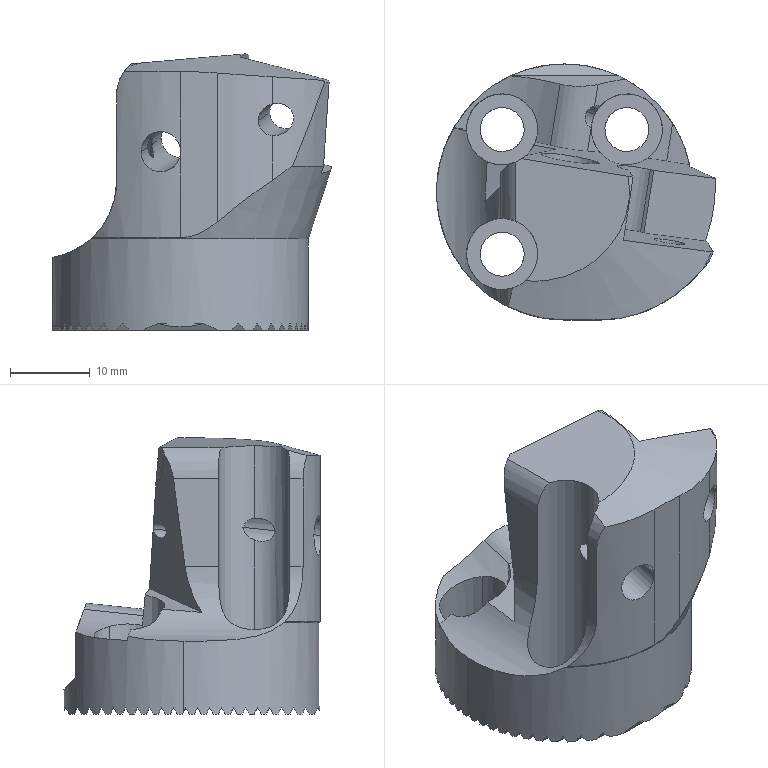CAM job | Mastercam | 3-axis milling, 5-axis milling, drilling
Tools:
tool_number,name,type,diameter_mm,corner_radius_mm,flutes,flute_length_mm,overall_length_mm,shoulder_length_mm,holder_diameter_mm,length_offset,diameter_offset,default_rpm,default_feed_mm_min,default_plunge_mm_min,coolant
1,2 Drill,drill,2,0,2,25,25,25,50,1,1,2998,359.76,600,COOL_OFF
2,6 120deg Spot Drill,drill,6,0,2,25,35,35,31.877,2,2,1000,120,600,COOL_OFF
3,4.3 Drill,drill,4.3,0,2,25,40,40,31.877,3,3,1395,167.4,600,COOL_OFF
4,12 Flat End Mill Rough,end mill,12,0,4,35,35,35,31.877,4,4,833,99.96,600,COOL_OFF
5,6 Flat End Mill Rough,end mill,6,0,4,20,20,20,31.877,5,5,1667,200.04,600,COOL_OFF
6,4 Flat End Mill Rough,end mill,4,0,4,20,20,20,27.495,6,6,2501,300.12,600,COOL_OFF
7,4 Flat End Mill Finish,end mill,4,0,4,20,20,20,27.495,7,7,2501,300.12,600,COOL_OFF
9,12 Flat End Mill Finish,end mill,12,0,4,35,35,35,31.877,9,9,833,99.96,600,COOL_OFF
10,30 Bull Nose Mill,bull end mill,30,0.8,4,25,50,25,50,10,10,400,48,600,COOL_OFF
11,4 Flat End Mill,end mill,4,0,4,20,20,20,50,11,11,2222,266.64,600,COOL_OFF
12,6 Spot Drill,drill,6,0,2,25,50,37,50,12,12,1000,120,600,COOL_OFF
13,3.3 Drill,drill,3.3,0,2,25,50,40,50,13,13,1818,218.16,600,COOL_OFF
14,3.15 Thread Mill,thread mill,3.15,0,4,2.1,20,20,31.877,14,14,1905,228.6,600,COOL_OFF
15,2.5 Ball Mill,ball end mill,2.5,1.25,4,3,20,3,31.877,15,15,4800,576,600,COOL_OFF
16,M5 x 0.8 RH Tap,drill,5,0,2,22,25,22,31.877,16,16,1200,960.0,600,COOL_OFF
17,3 Drill,drill,3,0,2,25,40,35,50,17,17,2000,240,600,COOL_OFF
18,5.5 Flat Mill,end mill,5.5,0,4,25,25,25,50,18,18,1818,218.16,600,COOL_OFF
Operations:
seq,operation,operation_type,tool_number,tool_name,tool_diameter_mm,spindle_rpm,feed_mm_min,plunge_mm_min,retract_mm_min,cycle_time_s,wcs,posted,nc_file
1,2D High Speed (2D Dynamic Mill) - [WCS: Top] - [Tplane: Top],HighSpeed2D,4,12 Flat End Mill Rough,12,3500,2500,2000,1200,17.289,Top,yes,.nc
2,2D High Speed (2D Dynamic Mill) - [WCS: Top] - [Tplane: Ins],HighSpeed2D,4,12 Flat End Mill Rough,12,3500,2500,2000,1200,118.677,Top,yes,.nc
3,Contour (2D) - [WCS: Top] - [Tplane: Ins],Contour,4,12 Flat End Mill Rough,12,3500,1000,2000,1200,7.025,Top,yes,.nc
4,Contour (Ramp) - [WCS: Top] - [Tplane: A0],Contour,4,12 Flat End Mill Rough,12,3500,1000,2000,1200,6.229,Top,yes,.nc
5,Contour (Ramp) - [WCS: Top] - [Tplane: A45],Contour,4,12 Flat End Mill Rough,12,3500,1000,2000,1200,4.179,Top,yes,.nc
6,Contour (Ramp) - [WCS: Top] - [Tplane: A-30],Contour,4,12 Flat End Mill Rough,12,3500,1000,2000,1200,4.291,Top,yes,.nc
7,2D High Speed (2D Dynamic Mill) - [WCS: Top] - [Tplane: A0-1],HighSpeed2D,4,12 Flat End Mill Rough,12,3500,2500,2000,1200,44.017,Top,yes,.nc
8,2D High Speed (2D Dynamic Mill) - [WCS: Top] - [Tplane: Ins],HighSpeed2D,5,6 Flat End Mill Rough,6,3500,1500,2000,1200,72.03,Top,yes,.nc
9,Contour (Remachining) - [WCS: Top] - [Tplane: Ins],Contour,6,4 Flat End Mill Rough,4,3500,400,2000,1200,68.934,Top,yes,.nc
10,Contour (Ramp) - [WCS: Top] - [Tplane: Ins],Contour,6,4 Flat End Mill Rough,4,3500,400,2000,1200,25.066,Top,yes,.nc
11,Contour (2D) - [WCS: Top] - [Tplane: Ins],Contour,7,4 Flat End Mill Finish,4,3500,400,2000,1200,16.515,Top,yes,.nc
12,Contour (2D) - [WCS: Top] - [Tplane: Pl-2],Contour,7,4 Flat End Mill Finish,4,3500,400,2000,1200,2.3,Top,yes,.nc
13,Contour (2D) - [WCS: Top] - [Tplane: Pl-3],Contour,7,4 Flat End Mill Finish,4,3500,400,2000,1200,2.316,Top,yes,.nc
14,Contour (2D) - [WCS: Top] - [Tplane: Top],Contour,9,12 Flat End Mill Finish,12,3500,600,2000,1200,16.491,Top,yes,.nc
15,Contour (2D) - [WCS: Top] - [Tplane: Ins],Contour,9,12 Flat End Mill Finish,12,3500,600,2000,1200,5.685,Top,yes,.nc
16,Contour (2D) - [WCS: Top] - [Tplane: A0],Contour,9,12 Flat End Mill Finish,12,3500,600,2000,1200,3.71,Top,yes,.nc
17,Contour (2D) - [WCS: Top] - [Tplane: A45],Contour,9,12 Flat End Mill Finish,12,3500,600,2000,1200,3.552,Top,yes,.nc
18,Contour (2D) - [WCS: Top] - [Tplane: A-30],Contour,9,12 Flat End Mill Finish,12,3500,600,2000,1200,3.664,Top,yes,.nc
19,Contour (2D) - [WCS: Top] - [Tplane: A0-1],Contour,9,12 Flat End Mill Finish,12,3500,600,2000,1200,6.75,Top,yes,.nc
20,Contour (2D) - [WCS: Top] - [Tplane: Ins],Contour,10,30 Bull Nose Mill,30,3500,400,2000,1200,11.272,Top,yes,.nc
21,Drill/Counterbore - [WCS: Top] - [Tplane: A0],Drill,12,6 Spot Drill,6,2000,100,5.409,5.409,1.68,Top,yes,.nc
22,Drill/Counterbore - [WCS: Top] - [Tplane: Ins],Drill,12,6 Spot Drill,6,2000,100,5.409,5.409,5.052,Top,yes,.nc
23,Peck Drill - [WCS: Top] - [Tplane: Ins],Drill,3,4.3 Drill,4.3,2500,100,600,1200,12.631,Top,yes,.nc
24,Peck Drill - [WCS: Top] - [Tplane: Ins],Drill,13,3.3 Drill,3.3,3000,60,600,1200,12.632,Top,yes,.nc
25,Peck Drill - [WCS: Top] - [Tplane: A0],Drill,13,3.3 Drill,3.3,3000,60,600,1200,13.763,Top,yes,.nc
26,Drill/Counterbore - [WCS: Top] - [Tplane: Ins],Drill,1,2 Drill,2,3000,60,600,1200,7.093,Top,yes,.nc
27,Drill/Counterbore - [WCS: Top] - [Tplane: CB],Drill,11,4 Flat End Mill,4,2000,100,600,1200,3.486,Top,yes,.nc
28,Drill/Counterbore - [WCS: Top] - [Tplane: CB],Drill,18,5.5 Flat Mill,5.5,1000,100,600,1200,4.09,Top,yes,.nc
29,Drill/Counterbore - [WCS: Top] - [Tplane: Ins],Drill,12,6 Spot Drill,6,2000,200,600,1200,1.559,Top,yes,.nc
30,Drill/Counterbore - [WCS: Top] - [Tplane: Ins],Drill,12,6 Spot Drill,6,2000,200,600,1200,1.407,Top,yes,.nc
31,Drill/Counterbore - [WCS: Top] - [Tplane: A0],Drill,12,6 Spot Drill,6,2000,200,600,1200,1.415,Top,yes,.nc
32,Thread Mill - [WCS: Top] - [Tplane: A0],ThreadMill,14,3.15 Thread Mill,3.15,3000,300,2000,1200,7.04,Top,yes,.nc
33,Stock model - [WCS: Top] - [Tplane: Top] - 2,139,,,,0,0,0,0,0,Top,no,
34,Thread Mill - [WCS: Top] - [Tplane: Ins],ThreadMill,14,3.15 Thread Mill,3.15,3000,300,2000,1200,22.324,Top,yes,.nc
35,Tap - [WCS: Top] - [Tplane: Ins],Drill,16,M5 x 0.8 RH Tap,5,200,160.0,600,1200,25.356,Top,yes,.nc
36,2D High Speed (2D Dynamic Mill) - [WCS: Top] - [Tplane: BkB],HighSpeed2D,4,12 Flat End Mill Rough,12,3500,2000,2000,1200,12.497,Top,yes,.nc
37,Contour (2D) - [WCS: Top] - [Tplane: BkB],Contour,9,12 Flat End Mill Finish,12,3500,600,2000,1200,2.75,Top,yes,.nc
38,Deburr 5-axis - [WCS: Top] - [Tplane: Top],459,15,2.5 Ball Mill,2.5,4500,1000,600,1200,7.913,Top,yes,.nc
39,Deburr 5-axis - [WCS: Top] - [Tplane: Top],459,15,2.5 Ball Mill,2.5,4500,1000,600,1200,4.558,Top,yes,.nc
40,Drill/Counterbore - [WCS: Top] - [Tplane: Outlet hole],Drill,2,6 120deg Spot Drill,6,2000,80,600,1200,2.361,Top,yes,.nc
41,Drill/Counterbore - [WCS: Top] - [Tplane: Outlet hole],Drill,17,3 Drill,3,2000,10,600,1200,48.354,Top,yes,.nc
42,Swarf machining - [WCS: Top] - [Tplane: Ins],441,7,4 Flat End Mill Finish,4,2501,300.12,600,1200,0,Top,no,
43,Swarf machining - [WCS: Top] - [Tplane: Top],441,7,4 Flat End Mill Finish,4,2501,300.12,600,1200,0,Top,no,